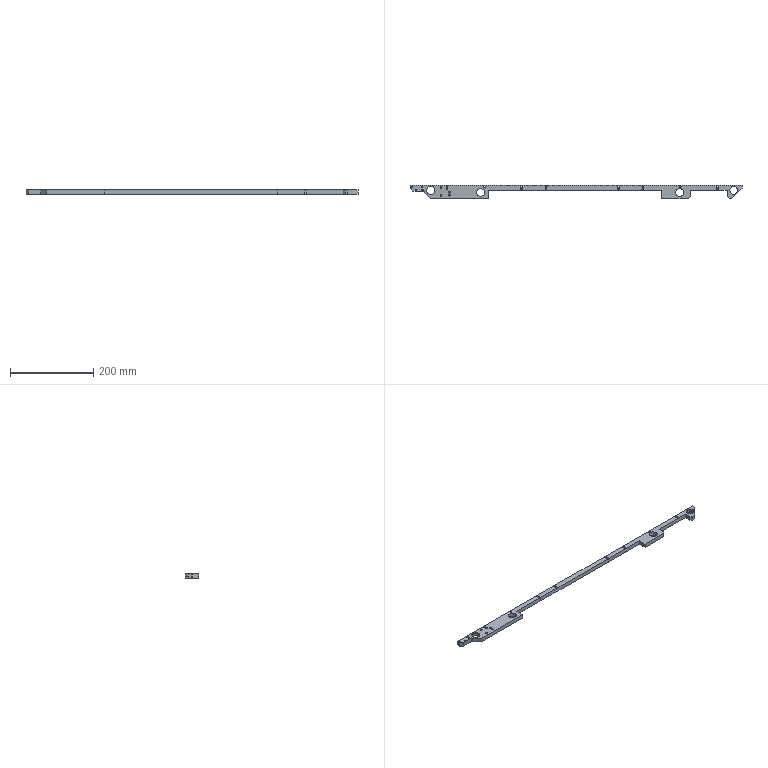Part | NX | 1 solid | 192 faces | box 800 x 32 x 10 mm | volume 127934 mm3 | cylinder 108 | cone 60 | plane 24 | commonest cylinder face diameters 2.5 x48 4 x20 4.5 x10 3.5 x6 4.63 x6 19 x6